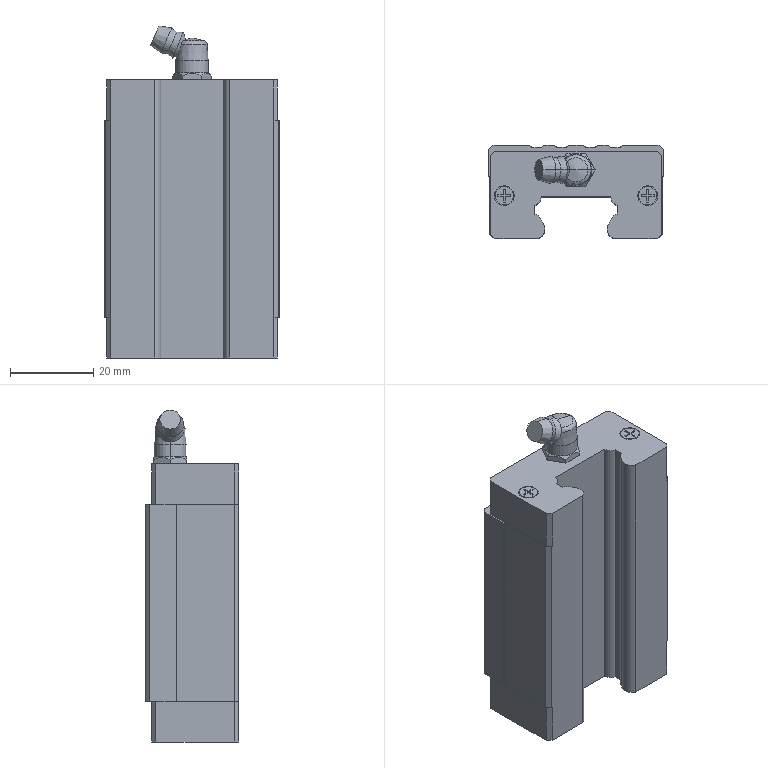Part | SolidWorks | features BaseBody 1 | 1 solid | 187 faces | box 42 x 22.5 x 80 mm | volume 49279 mm3 | plane 94 | cylinder 61 | cone 30 | spline 2 | commonest cylinder face diameters 3.08 x20 2 x8 4.134 x8 4.4 x8 4.8 x8 4.2 x4